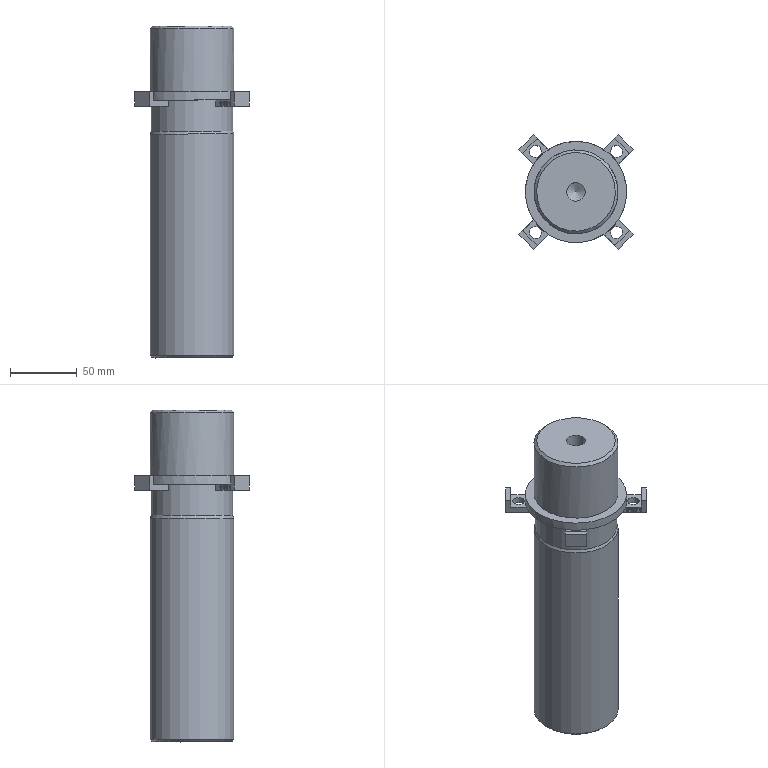Part | STEP file | gslz 2016.10.28-10_id174_x_t | 1 solid | 228 faces | box 85.913 x 85.913 x 249 mm | volume 777176 mm3 | plane 136 | other 76 | cylinder 10 | cone 5 | torus 1 | commonest cylinder face diameters 9 x4 63 x2 8.5 x1 14 x1 61 x1 76 x1